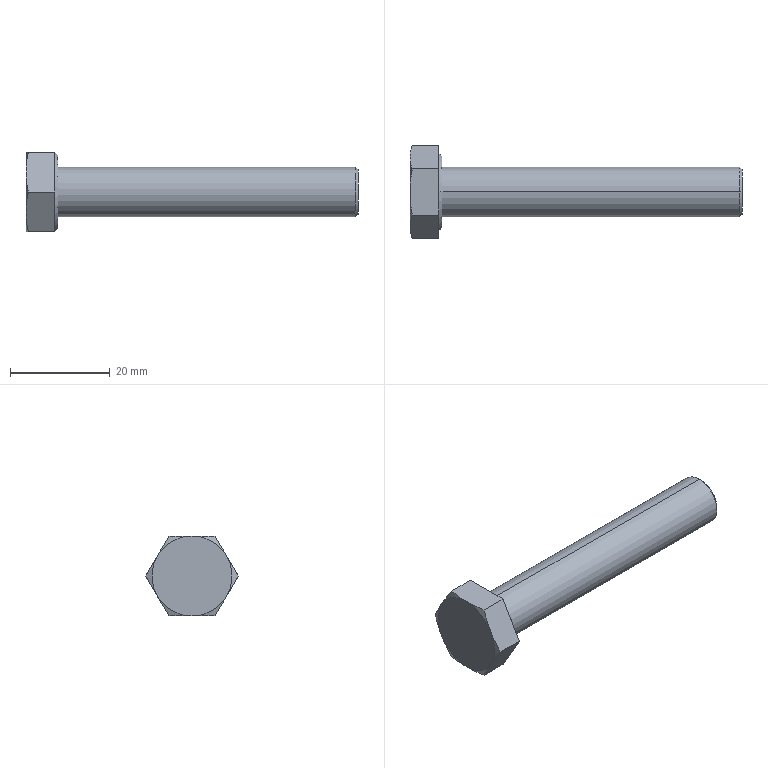Part | SolidWorks | features BaseBody 1 | 1 solid | 22 faces | box 66.4 x 18.475 x 16 mm | volume 6099 mm3 | cone 10 | plane 10 | cylinder 2 | commonest cylinder face diameters 10 x2
STEP:
#1=CARTESIAN_POINT('',(65.9,0.,5.));
#2=VERTEX_POINT('',#1);
#3=CARTESIAN_POINT('',(65.9,0.,-5.));
#4=VERTEX_POINT('',#3);
#5=CARTESIAN_POINT('',(65.9,0.,0.));
#6=DIRECTION('',(-1.,0.,0.));
#7=DIRECTION('',(0.,0.,1.));
#8=AXIS2_PLACEMENT_3D('',#5,#6,#7);
#9=CIRCLE('',#8,5.);
#10=EDGE_CURVE('',#2,#4,#9,.T.);
#11=ORIENTED_EDGE('',*,*,#10,.T.);
#12=CARTESIAN_POINT('',(6.4,0.,-5.));
#13=VERTEX_POINT('',#12);
#14=CARTESIAN_POINT('',(66.4,0.,-5.));
#15=DIRECTION('',(-1.,0.,0.));
#16=VECTOR('',#15,1000.);
#17=LINE('',#14,#16);
#18=EDGE_CURVE('',#4,#13,#17,.T.);
#19=ORIENTED_EDGE('',*,*,#18,.T.);
#20=CARTESIAN_POINT('',(6.4,0.,5.));
#21=VERTEX_POINT('',#20);
#22=CARTESIAN_POINT('',(6.4,0.,0.));
#23=DIRECTION('',(1.,0.,0.));
#24=DIRECTION('',(0.,0.,1.));
#25=AXIS2_PLACEMENT_3D('',#22,#23,#24);
#26=CIRCLE('',#25,5.);
#27=EDGE_CURVE('',#13,#21,#26,.T.);
#28=ORIENTED_EDGE('',*,*,#27,.T.);
#29=CARTESIAN_POINT('',(66.4,0.,5.));
#30=DIRECTION('',(-1.,0.,0.));
#31=VECTOR('',#30,1000.);
#32=LINE('',#29,#31);
#33=EDGE_CURVE('',#2,#21,#32,.T.);
#34=ORIENTED_EDGE('',*,*,#33,.F.);
#35=EDGE_LOOP('',(#11,#19,#28,#34));
#36=FACE_OUTER_BOUND('',#35,.T.);
#37=CARTESIAN_POINT('',(66.4,0.,0.));
#38=DIRECTION('',(-1.,0.,0.));
#39=DIRECTION('',(0.,0.,1.));
#40=AXIS2_PLACEMENT_3D('',#37,#38,#39);
#41=CYLINDRICAL_SURFACE('',#40,5.);
#42=ADVANCED_FACE('',(#36),#41,.T.);
#43=CARTESIAN_POINT('',(66.4,0.,4.5));
#44=VERTEX_POINT('',#43);
#45=CARTESIAN_POINT('',(66.4,0.,-4.5));
#46=VERTEX_POINT('',#45);
#47=CARTESIAN_POINT('',(66.4,0.,0.));
#48=DIRECTION('',(-1.,0.,0.));
#49=DIRECTION('',(0.,0.,1.));
#50=AXIS2_PLACEMENT_3D('',#47,#48,#49);
#51=CIRCLE('',#50,4.5);
#52=EDGE_CURVE('',#44,#46,#51,.T.);
#53=ORIENTED_EDGE('',*,*,#52,.T.);
#54=CARTESIAN_POINT('',(65.9,0.,-5.));
#55=DIRECTION('',(-0.7071,0.,-0.7071));
#56=VECTOR('',#55,1000.);
#57=LINE('',#54,#56);
#58=EDGE_CURVE('',#46,#4,#57,.T.);
#59=ORIENTED_EDGE('',*,*,#58,.T.);
#60=ORIENTED_EDGE('',*,*,#10,.F.);
#61=CARTESIAN_POINT('',(65.9,0.,5.));
#62=DIRECTION('',(-0.7071,0.,0.7071));
#63=VECTOR('',#62,1000.);
#64=LINE('',#61,#63);
#65=EDGE_CURVE('',#44,#2,#64,.T.);
#66=ORIENTED_EDGE('',*,*,#65,.F.);
#67=EDGE_LOOP('',(#53,#59,#60,#66));
#68=FACE_OUTER_BOUND('',#67,.T.);
#69=CARTESIAN_POINT('',(65.9,0.,0.));
#70=DIRECTION('',(-1.,0.,0.));
#71=DIRECTION('',(0.,0.,1.));
#72=AXIS2_PLACEMENT_3D('',#69,#70,#71);
#73=CONICAL_SURFACE('',#72,5.,0.7854);
#74=ADVANCED_FACE('',(#68),#73,.T.);
#75=CARTESIAN_POINT('',(6.4,0.,7.235));
#76=VERTEX_POINT('',#75);
#77=CARTESIAN_POINT('',(6.4,0.,-7.235));
#78=VERTEX_POINT('',#77);
#79=CARTESIAN_POINT('',(6.4,0.,0.));
#80=DIRECTION('',(-1.,0.,0.));
#81=DIRECTION('',(0.,0.,1.));
#82=AXIS2_PLACEMENT_3D('',#79,#80,#81);
#83=CIRCLE('',#82,7.235);
#84=EDGE_CURVE('',#76,#78,#83,.T.);
#85=ORIENTED_EDGE('',*,*,#84,.T.);
#86=CARTESIAN_POINT('',(5.8,0.,-7.835));
#87=VERTEX_POINT('',#86);
#88=CARTESIAN_POINT('',(5.8,0.,-7.835));
#89=DIRECTION('',(-0.7071,0.,-0.7071));
#90=VECTOR('',#89,1000.);
#91=LINE('',#88,#90);
#92=EDGE_CURVE('',#78,#87,#91,.T.);
#93=ORIENTED_EDGE('',*,*,#92,.T.);
#94=CARTESIAN_POINT('',(5.8,0.,7.835));
#95=VERTEX_POINT('',#94);
#96=CARTESIAN_POINT('',(5.8,0.,0.));
#97=DIRECTION('',(1.,0.,0.));
#98=DIRECTION('',(0.,0.,1.));
#99=AXIS2_PLACEMENT_3D('',#96,#97,#98);
#100=CIRCLE('',#99,7.835);
#101=EDGE_CURVE('',#87,#95,#100,.T.);
#102=ORIENTED_EDGE('',*,*,#101,.T.);
#103=CARTESIAN_POINT('',(5.8,0.,7.835));
#104=DIRECTION('',(-0.7071,0.,0.7071));
#105=VECTOR('',#104,1000.);
#106=LINE('',#103,#105);
#107=EDGE_CURVE('',#76,#95,#106,.T.);
#108=ORIENTED_EDGE('',*,*,#107,.F.);
#109=EDGE_LOOP('',(#85,#93,#102,#108));
#110=FACE_OUTER_BOUND('',#109,.T.);
#111=CARTESIAN_POINT('',(5.8,0.,0.));
#112=DIRECTION('',(-1.,0.,0.));
#113=DIRECTION('',(0.,0.,1.));
#114=AXIS2_PLACEMENT_3D('',#111,#112,#113);
#115=CONICAL_SURFACE('',#114,7.835,0.7854);
#116=ADVANCED_FACE('',(#110),#115,.T.);
#117=ORIENTED_EDGE('',*,*,#18,.F.);
#118=CARTESIAN_POINT('',(65.9,0.,0.));
#119=DIRECTION('',(-1.,0.,0.));
#120=DIRECTION('',(0.,0.,1.));
#121=AXIS2_PLACEMENT_3D('',#118,#119,#120);
#122=CIRCLE('',#121,5.);
#123=EDGE_CURVE('',#4,#2,#122,.T.);
#124=ORIENTED_EDGE('',*,*,#123,.T.);
#125=ORIENTED_EDGE('',*,*,#33,.T.);
#126=CARTESIAN_POINT('',(6.4,0.,0.));
#127=DIRECTION('',(1.,0.,0.));
#128=DIRECTION('',(0.,0.,1.));
#129=AXIS2_PLACEMENT_3D('',#126,#127,#128);
#130=CIRCLE('',#129,5.);
#131=EDGE_CURVE('',#21,#13,#130,.T.);
#132=ORIENTED_EDGE('',*,*,#131,.T.);
#133=EDGE_LOOP('',(#117,#124,#125,#132));
#134=FACE_OUTER_BOUND('',#133,.T.);
#135=CARTESIAN_POINT('',(66.4,0.,0.));
#136=DIRECTION('',(-1.,0.,0.));
#137=DIRECTION('',(0.,0.,1.));
#138=AXIS2_PLACEMENT_3D('',#135,#136,#137);
#139=CYLINDRICAL_SURFACE('',#138,5.);
#140=ADVANCED_FACE('',(#134),#139,.T.);
#141=ORIENTED_EDGE('',*,*,#131,.F.);
#142=ORIENTED_EDGE('',*,*,#27,.F.);
#143=EDGE_LOOP('',(#141,#142));
#144=FACE_BOUND('',#143,.T.);
#145=ORIENTED_EDGE('',*,*,#84,.F.);
#146=CARTESIAN_POINT('',(6.4,0.,0.));
#147=DIRECTION('',(-1.,0.,0.));
#148=DIRECTION('',(0.,0.,1.));
#149=AXIS2_PLACEMENT_3D('',#146,#147,#148);
#150=CIRCLE('',#149,7.235);
#151=EDGE_CURVE('',#78,#76,#150,.T.);
#152=ORIENTED_EDGE('',*,*,#151,.F.);
#153=EDGE_LOOP('',(#145,#152));
#154=FACE_OUTER_BOUND('',#153,.T.);
#155=CARTESIAN_POINT('',(6.4,-4.619,8.));
#156=DIRECTION('',(-1.,0.,0.));
#157=DIRECTION('',(0.,0.,1.));
#158=AXIS2_PLACEMENT_3D('',#155,#156,#157);
#159=PLANE('',#158);
#160=ADVANCED_FACE('',(#144,#154),#159,.F.);
#161=ORIENTED_EDGE('',*,*,#58,.F.);
#162=CARTESIAN_POINT('',(66.4,0.,0.));
#163=DIRECTION('',(-1.,0.,0.));
#164=DIRECTION('',(0.,0.,1.));
#165=AXIS2_PLACEMENT_3D('',#162,#163,#164);
#166=CIRCLE('',#165,4.5);
#167=EDGE_CURVE('',#46,#44,#166,.T.);
#168=ORIENTED_EDGE('',*,*,#167,.T.);
#169=ORIENTED_EDGE('',*,*,#65,.T.);
#170=ORIENTED_EDGE('',*,*,#123,.F.);
#171=EDGE_LOOP('',(#161,#168,#169,#170));
#172=FACE_OUTER_BOUND('',#171,.T.);
#173=CARTESIAN_POINT('',(65.9,0.,0.));
#174=DIRECTION('',(-1.,0.,0.));
#175=DIRECTION('',(0.,0.,1.));
#176=AXIS2_PLACEMENT_3D('',#173,#174,#175);
#177=CONICAL_SURFACE('',#176,5.,0.7854);
#178=ADVANCED_FACE('',(#172),#177,.T.);
#179=ORIENTED_EDGE('',*,*,#92,.F.);
#180=ORIENTED_EDGE('',*,*,#151,.T.);
#181=ORIENTED_EDGE('',*,*,#107,.T.);
#182=CARTESIAN_POINT('',(5.8,0.,0.));
#183=DIRECTION('',(1.,0.,0.));
#184=DIRECTION('',(0.,0.,1.));
#185=AXIS2_PLACEMENT_3D('',#182,#183,#184);
#186=CIRCLE('',#185,7.835);
#187=EDGE_CURVE('',#95,#87,#186,.T.);
#188=ORIENTED_EDGE('',*,*,#187,.T.);
#189=EDGE_LOOP('',(#179,#180,#181,#188));
#190=FACE_OUTER_BOUND('',#189,.T.);
#191=CARTESIAN_POINT('',(5.8,0.,0.));
#192=DIRECTION('',(-1.,0.,0.));
#193=DIRECTION('',(0.,0.,1.));
#194=AXIS2_PLACEMENT_3D('',#191,#192,#193);
#195=CONICAL_SURFACE('',#194,7.835,0.7854);
#196=ADVANCED_FACE('',(#190),#195,.T.);
#197=ORIENTED_EDGE('',*,*,#52,.F.);
#198=ORIENTED_EDGE('',*,*,#167,.F.);
#199=EDGE_LOOP('',(#197,#198));
#200=FACE_OUTER_BOUND('',#199,.T.);
#201=CARTESIAN_POINT('',(66.4,0.,0.));
#202=DIRECTION('',(1.,0.,0.));
#203=DIRECTION('',(0.,0.,-1.));
#204=AXIS2_PLACEMENT_3D('',#201,#202,#203);
#205=PLANE('',#204);
#206=ADVANCED_FACE('',(#200),#205,.T.);
#207=CARTESIAN_POINT('',(5.8,9.238,0.));
#208=VERTEX_POINT('',#207);
#209=CARTESIAN_POINT('',(5.8,4.619,8.));
#210=VERTEX_POINT('',#209);
#211=CARTESIAN_POINT('',(5.8,9.238,0.));
#212=DIRECTION('',(0.,-0.5,0.866));
#213=VECTOR('',#212,1000.);
#214=LINE('',#211,#213);
#215=EDGE_CURVE('',#208,#210,#214,.T.);
#216=ORIENTED_EDGE('',*,*,#215,.T.);
#217=CARTESIAN_POINT('',(5.8,-4.619,8.));
#218=VERTEX_POINT('',#217);
#219=CARTESIAN_POINT('',(5.8,7.835,8.));
#220=DIRECTION('',(0.,-1.,0.));
#221=VECTOR('',#220,1000.);
#222=LINE('',#219,#221);
#223=EDGE_CURVE('',#210,#218,#222,.T.);
#224=ORIENTED_EDGE('',*,*,#223,.T.);
#225=CARTESIAN_POINT('',(5.8,-9.238,0.));
#226=VERTEX_POINT('',#225);
#227=CARTESIAN_POINT('',(5.8,-4.619,8.));
#228=DIRECTION('',(0.,-0.5,-0.866));
#229=VECTOR('',#228,1000.);
#230=LINE('',#227,#229);
#231=EDGE_CURVE('',#218,#226,#230,.T.);
#232=ORIENTED_EDGE('',*,*,#231,.T.);
#233=CARTESIAN_POINT('',(5.8,-4.619,-8.));
#234=VERTEX_POINT('',#233);
#235=CARTESIAN_POINT('',(5.8,-9.238,0.));
#236=DIRECTION('',(0.,0.5,-0.866));
#237=VECTOR('',#236,1000.);
#238=LINE('',#235,#237);
#239=EDGE_CURVE('',#226,#234,#238,.T.);
#240=ORIENTED_EDGE('',*,*,#239,.T.);
#241=CARTESIAN_POINT('',(5.8,4.619,-8.));
#242=VERTEX_POINT('',#241);
#243=CARTESIAN_POINT('',(5.8,7.835,-8.));
#244=DIRECTION('',(0.,1.,0.));
#245=VECTOR('',#244,1000.);
#246=LINE('',#243,#245);
#247=EDGE_CURVE('',#234,#242,#246,.T.);
#248=ORIENTED_EDGE('',*,*,#247,.T.);
#249=CARTESIAN_POINT('',(5.8,4.619,-8.));
#250=DIRECTION('',(0.,0.5,0.866));
#251=VECTOR('',#250,1000.);
#252=LINE('',#249,#251);
#253=EDGE_CURVE('',#242,#208,#252,.T.);
#254=ORIENTED_EDGE('',*,*,#253,.T.);
#255=EDGE_LOOP('',(#216,#224,#232,#240,#248,#254));
#256=FACE_OUTER_BOUND('',#255,.T.);
#257=ORIENTED_EDGE('',*,*,#187,.F.);
#258=ORIENTED_EDGE('',*,*,#101,.F.);
#259=EDGE_LOOP('',(#257,#258));
#260=FACE_BOUND('',#259,.T.);
#261=CARTESIAN_POINT('',(5.8,7.835,0.));
#262=DIRECTION('',(1.,0.,0.));
#263=DIRECTION('',(0.,0.,-1.));
#264=AXIS2_PLACEMENT_3D('',#261,#262,#263);
#265=PLANE('',#264);
#266=ADVANCED_FACE('',(#256,#260),#265,.T.);
#267=CARTESIAN_POINT('',(0.4505,-4.619,8.));
#268=VERTEX_POINT('',#267);
#269=CARTESIAN_POINT('',(6.4,-4.619,8.));
#270=DIRECTION('',(-1.,0.,0.));
#271=VECTOR('',#270,1000.);
#272=LINE('',#269,#271);
#273=EDGE_CURVE('',#218,#268,#272,.T.);
#274=ORIENTED_EDGE('',*,*,#273,.F.);
#275=ORIENTED_EDGE('',*,*,#223,.F.);
#276=CARTESIAN_POINT('',(0.4505,4.619,8.));
#277=VERTEX_POINT('',#276);
#278=CARTESIAN_POINT('',(6.4,4.619,8.));
#279=DIRECTION('',(1.,0.,0.));
#280=VECTOR('',#279,1000.);
#281=LINE('',#278,#280);
#282=EDGE_CURVE('',#277,#210,#281,.T.);
#283=ORIENTED_EDGE('',*,*,#282,.F.);
#284=CARTESIAN_POINT('',(0.,0.,8.));
#285=VERTEX_POINT('',#284);
#286=CARTESIAN_POINT('',(0.,0.,8.));
#287=CARTESIAN_POINT('',(0.,0.7771,8.));
#288=CARTESIAN_POINT('',(0.04194,1.55,8.));
#289=CARTESIAN_POINT('',(0.1979,3.089,8.));
#290=CARTESIAN_POINT('',(0.3115,3.855,8.));
#291=CARTESIAN_POINT('',(0.4505,4.619,8.));
#292=B_SPLINE_CURVE_WITH_KNOTS('',3,(#286,#287,#288,#289,#290,#291),.UNSPECIFIED.,.F.,.F.,(4,2,4),(0.,0.00232,0.004641),.UNSPECIFIED.);
#293=EDGE_CURVE('',#285,#277,#292,.T.);
#294=ORIENTED_EDGE('',*,*,#293,.F.);
#295=CARTESIAN_POINT('',(0.4505,-4.619,8.));
#296=CARTESIAN_POINT('',(0.3115,-3.855,8.));
#297=CARTESIAN_POINT('',(0.1979,-3.089,8.));
#298=CARTESIAN_POINT('',(0.04194,-1.55,8.));
#299=CARTESIAN_POINT('',(0.,-0.7771,8.));
#300=CARTESIAN_POINT('',(0.,0.,8.));
#301=B_SPLINE_CURVE_WITH_KNOTS('',3,(#295,#296,#297,#298,#299,#300),.UNSPECIFIED.,.F.,.F.,(4,2,4),(0.,0.00232,0.004641),.UNSPECIFIED.);
#302=EDGE_CURVE('',#268,#285,#301,.T.);
#303=ORIENTED_EDGE('',*,*,#302,.F.);
#304=EDGE_LOOP('',(#274,#275,#283,#294,#303));
#305=FACE_OUTER_BOUND('',#304,.T.);
#306=CARTESIAN_POINT('',(6.4,4.619,8.));
#307=DIRECTION('',(0.,0.,-1.));
#308=DIRECTION('',(-1.,0.,0.));
#309=AXIS2_PLACEMENT_3D('',#306,#307,#308);
#310=PLANE('',#309);
#311=ADVANCED_FACE('',(#305),#310,.F.);
#312=ORIENTED_EDGE('',*,*,#282,.T.);
#313=ORIENTED_EDGE('',*,*,#215,.F.);
#314=CARTESIAN_POINT('',(0.4505,9.238,0.));
#315=VERTEX_POINT('',#314);
#316=CARTESIAN_POINT('',(6.4,9.238,0.));
#317=DIRECTION('',(1.,0.,0.));
#318=VECTOR('',#317,1000.);
#319=LINE('',#316,#318);
#320=EDGE_CURVE('',#315,#208,#319,.T.);
#321=ORIENTED_EDGE('',*,*,#320,.F.);
#322=CARTESIAN_POINT('',(0.,6.928,4.));
#323=VERTEX_POINT('',#322);
#324=CARTESIAN_POINT('',(0.,6.928,4.));
#325=CARTESIAN_POINT('',(0.,7.317,3.327));
#326=CARTESIAN_POINT('',(0.04194,7.703,2.658));
#327=CARTESIAN_POINT('',(0.1979,8.473,1.325));
#328=CARTESIAN_POINT('',(0.3115,8.856,0.6613));
#329=CARTESIAN_POINT('',(0.4505,9.238,0.));
#330=B_SPLINE_CURVE_WITH_KNOTS('',3,(#324,#325,#326,#327,#328,#329),.UNSPECIFIED.,.F.,.F.,(4,2,4),(0.,0.00232,0.004641),.UNSPECIFIED.);
#331=EDGE_CURVE('',#323,#315,#330,.T.);
#332=ORIENTED_EDGE('',*,*,#331,.F.);
#333=CARTESIAN_POINT('',(0.4505,4.619,8.));
#334=CARTESIAN_POINT('',(0.3115,5.001,7.339));
#335=CARTESIAN_POINT('',(0.1979,5.384,6.675));
#336=CARTESIAN_POINT('',(0.04194,6.153,5.342));
#337=CARTESIAN_POINT('',(0.,6.54,4.673));
#338=CARTESIAN_POINT('',(0.,6.928,4.));
#339=B_SPLINE_CURVE_WITH_KNOTS('',3,(#333,#334,#335,#336,#337,#338),.UNSPECIFIED.,.F.,.F.,(4,2,4),(0.,0.00232,0.004641),.UNSPECIFIED.);
#340=EDGE_CURVE('',#277,#323,#339,.T.);
#341=ORIENTED_EDGE('',*,*,#340,.F.);
#342=EDGE_LOOP('',(#312,#313,#321,#332,#341));
#343=FACE_OUTER_BOUND('',#342,.T.);
#344=CARTESIAN_POINT('',(6.4,9.238,0.));
#345=DIRECTION('',(0.,-0.866,-0.5));
#346=DIRECTION('',(0.,0.5,-0.866));
#347=AXIS2_PLACEMENT_3D('',#344,#345,#346);
#348=PLANE('',#347);
#349=ADVANCED_FACE('',(#343),#348,.F.);
#350=ORIENTED_EDGE('',*,*,#320,.T.);
#351=ORIENTED_EDGE('',*,*,#253,.F.);
#352=CARTESIAN_POINT('',(0.4505,4.619,-8.));
#353=VERTEX_POINT('',#352);
#354=CARTESIAN_POINT('',(6.4,4.619,-8.));
#355=DIRECTION('',(1.,0.,0.));
#356=VECTOR('',#355,1000.);
#357=LINE('',#354,#356);
#358=EDGE_CURVE('',#353,#242,#357,.T.);
#359=ORIENTED_EDGE('',*,*,#358,.F.);
#360=CARTESIAN_POINT('',(0.,6.928,-4.));
#361=VERTEX_POINT('',#360);
#362=CARTESIAN_POINT('',(0.,6.928,-4.));
#363=CARTESIAN_POINT('',(0.,6.54,-4.673));
#364=CARTESIAN_POINT('',(0.04194,6.153,-5.342));
#365=CARTESIAN_POINT('',(0.1979,5.384,-6.675));
#366=CARTESIAN_POINT('',(0.3115,5.001,-7.339));
#367=CARTESIAN_POINT('',(0.4505,4.619,-8.));
#368=B_SPLINE_CURVE_WITH_KNOTS('',3,(#362,#363,#364,#365,#366,#367),.UNSPECIFIED.,.F.,.F.,(4,2,4),(0.,0.00232,0.004641),.UNSPECIFIED.);
#369=EDGE_CURVE('',#361,#353,#368,.T.);
#370=ORIENTED_EDGE('',*,*,#369,.F.);
#371=CARTESIAN_POINT('',(0.4505,9.238,0.));
#372=CARTESIAN_POINT('',(0.3115,8.856,-0.6613));
#373=CARTESIAN_POINT('',(0.1979,8.473,-1.325));
#374=CARTESIAN_POINT('',(0.04194,7.703,-2.658));
#375=CARTESIAN_POINT('',(0.,7.317,-3.327));
#376=CARTESIAN_POINT('',(0.,6.928,-4.));
#377=B_SPLINE_CURVE_WITH_KNOTS('',3,(#371,#372,#373,#374,#375,#376),.UNSPECIFIED.,.F.,.F.,(4,2,4),(0.,0.00232,0.004641),.UNSPECIFIED.);
#378=EDGE_CURVE('',#315,#361,#377,.T.);
#379=ORIENTED_EDGE('',*,*,#378,.F.);
#380=EDGE_LOOP('',(#350,#351,#359,#370,#379));
#381=FACE_OUTER_BOUND('',#380,.T.);
#382=CARTESIAN_POINT('',(6.4,4.619,-8.));
#383=DIRECTION('',(0.,-0.866,0.5));
#384=DIRECTION('',(0.,-0.5,-0.866));
#385=AXIS2_PLACEMENT_3D('',#382,#383,#384);
#386=PLANE('',#385);
#387=ADVANCED_FACE('',(#381),#386,.F.);
#388=ORIENTED_EDGE('',*,*,#358,.T.);
#389=ORIENTED_EDGE('',*,*,#247,.F.);
#390=CARTESIAN_POINT('',(0.4505,-4.619,-8.));
#391=VERTEX_POINT('',#390);
#392=CARTESIAN_POINT('',(6.4,-4.619,-8.));
#393=DIRECTION('',(1.,0.,0.));
#394=VECTOR('',#393,1000.);
#395=LINE('',#392,#394);
#396=EDGE_CURVE('',#391,#234,#395,.T.);
#397=ORIENTED_EDGE('',*,*,#396,.F.);
#398=CARTESIAN_POINT('',(0.,0.,-8.));
#399=VERTEX_POINT('',#398);
#400=CARTESIAN_POINT('',(0.,0.,-8.));
#401=CARTESIAN_POINT('',(0.,-0.7771,-8.));
#402=CARTESIAN_POINT('',(0.04194,-1.55,-8.));
#403=CARTESIAN_POINT('',(0.1979,-3.089,-8.));
#404=CARTESIAN_POINT('',(0.3115,-3.855,-8.));
#405=CARTESIAN_POINT('',(0.4505,-4.619,-8.));
#406=B_SPLINE_CURVE_WITH_KNOTS('',3,(#400,#401,#402,#403,#404,#405),.UNSPECIFIED.,.F.,.F.,(4,2,4),(0.,0.00232,0.004641),.UNSPECIFIED.);
#407=EDGE_CURVE('',#399,#391,#406,.T.);
#408=ORIENTED_EDGE('',*,*,#407,.F.);
#409=CARTESIAN_POINT('',(0.4505,4.619,-8.));
#410=CARTESIAN_POINT('',(0.3115,3.855,-8.));
#411=CARTESIAN_POINT('',(0.1979,3.089,-8.));
#412=CARTESIAN_POINT('',(0.04194,1.55,-8.));
#413=CARTESIAN_POINT('',(0.,0.7771,-8.));
#414=CARTESIAN_POINT('',(0.,0.,-8.));
#415=B_SPLINE_CURVE_WITH_KNOTS('',3,(#409,#410,#411,#412,#413,#414),.UNSPECIFIED.,.F.,.F.,(4,2,4),(0.,0.00232,0.004641),.UNSPECIFIED.);
#416=EDGE_CURVE('',#353,#399,#415,.T.);
#417=ORIENTED_EDGE('',*,*,#416,.F.);
#418=EDGE_LOOP('',(#388,#389,#397,#408,#417));
#419=FACE_OUTER_BOUND('',#418,.T.);
#420=CARTESIAN_POINT('',(6.4,-4.619,-8.));
#421=DIRECTION('',(0.,0.,1.));
#422=DIRECTION('',(1.,0.,0.));
#423=AXIS2_PLACEMENT_3D('',#420,#421,#422);
#424=PLANE('',#423);
#425=ADVANCED_FACE('',(#419),#424,.F.);
#426=ORIENTED_EDGE('',*,*,#396,.T.);
#427=ORIENTED_EDGE('',*,*,#239,.F.);
#428=CARTESIAN_POINT('',(0.4505,-9.238,0.));
#429=VERTEX_POINT('',#428);
#430=CARTESIAN_POINT('',(6.4,-9.238,0.));
#431=DIRECTION('',(1.,0.,0.));
#432=VECTOR('',#431,1000.);
#433=LINE('',#430,#432);
#434=EDGE_CURVE('',#429,#226,#433,.T.);
#435=ORIENTED_EDGE('',*,*,#434,.F.);
#436=CARTESIAN_POINT('',(0.,-6.928,-4.));
#437=VERTEX_POINT('',#436);
#438=CARTESIAN_POINT('',(0.,-6.928,-4.));
#439=CARTESIAN_POINT('',(0.,-7.317,-3.327));
#440=CARTESIAN_POINT('',(0.04194,-7.703,-2.658));
#441=CARTESIAN_POINT('',(0.1979,-8.473,-1.325));
#442=CARTESIAN_POINT('',(0.3115,-8.856,-0.6613));
#443=CARTESIAN_POINT('',(0.4505,-9.238,0.));
#444=B_SPLINE_CURVE_WITH_KNOTS('',3,(#438,#439,#440,#441,#442,#443),.UNSPECIFIED.,.F.,.F.,(4,2,4),(0.,0.00232,0.004641),.UNSPECIFIED.);
#445=EDGE_CURVE('',#437,#429,#444,.T.);
#446=ORIENTED_EDGE('',*,*,#445,.F.);
#447=CARTESIAN_POINT('',(0.4505,-4.619,-8.));
#448=CARTESIAN_POINT('',(0.3115,-5.001,-7.339));
#449=CARTESIAN_POINT('',(0.1979,-5.384,-6.675));
#450=CARTESIAN_POINT('',(0.04194,-6.153,-5.342));
#451=CARTESIAN_POINT('',(0.,-6.54,-4.673));
#452=CARTESIAN_POINT('',(0.,-6.928,-4.));
#453=B_SPLINE_CURVE_WITH_KNOTS('',3,(#447,#448,#449,#450,#451,#452),.UNSPECIFIED.,.F.,.F.,(4,2,4),(0.,0.00232,0.004641),.UNSPECIFIED.);
#454=EDGE_CURVE('',#391,#437,#453,.T.);
#455=ORIENTED_EDGE('',*,*,#454,.F.);
#456=EDGE_LOOP('',(#426,#427,#435,#446,#455));
#457=FACE_OUTER_BOUND('',#456,.T.);
#458=CARTESIAN_POINT('',(6.4,-9.238,0.));
#459=DIRECTION('',(0.,0.866,0.5));
#460=DIRECTION('',(0.,-0.5,0.866));
#461=AXIS2_PLACEMENT_3D('',#458,#459,#460);
#462=PLANE('',#461);
#463=ADVANCED_FACE('',(#457),#462,.F.);
#464=ORIENTED_EDGE('',*,*,#434,.T.);
#465=ORIENTED_EDGE('',*,*,#231,.F.);
#466=ORIENTED_EDGE('',*,*,#273,.T.);
#467=CARTESIAN_POINT('',(0.,-6.928,4.));
#468=VERTEX_POINT('',#467);
#469=CARTESIAN_POINT('',(0.,-6.928,4.));
#470=CARTESIAN_POINT('',(0.,-6.54,4.673));
#471=CARTESIAN_POINT('',(0.04194,-6.153,5.342));
#472=CARTESIAN_POINT('',(0.1979,-5.384,6.675));
#473=CARTESIAN_POINT('',(0.3115,-5.001,7.339));
#474=CARTESIAN_POINT('',(0.4505,-4.619,8.));
#475=B_SPLINE_CURVE_WITH_KNOTS('',3,(#469,#470,#471,#472,#473,#474),.UNSPECIFIED.,.F.,.F.,(4,2,4),(0.,0.00232,0.004641),.UNSPECIFIED.);
#476=EDGE_CURVE('',#468,#268,#475,.T.);
#477=ORIENTED_EDGE('',*,*,#476,.F.);
#478=CARTESIAN_POINT('',(0.4505,-9.238,0.));
#479=CARTESIAN_POINT('',(0.3115,-8.856,0.6613));
#480=CARTESIAN_POINT('',(0.1979,-8.473,1.325));
#481=CARTESIAN_POINT('',(0.04194,-7.703,2.658));
#482=CARTESIAN_POINT('',(0.,-7.317,3.327));
#483=CARTESIAN_POINT('',(0.,-6.928,4.));
#484=B_SPLINE_CURVE_WITH_KNOTS('',3,(#478,#479,#480,#481,#482,#483),.UNSPECIFIED.,.F.,.F.,(4,2,4),(0.,0.00232,0.004641),.UNSPECIFIED.);
#485=EDGE_CURVE('',#429,#468,#484,.T.);
#486=ORIENTED_EDGE('',*,*,#485,.F.);
#487=EDGE_LOOP('',(#464,#465,#466,#477,#486));
#488=FACE_OUTER_BOUND('',#487,.T.);
#489=CARTESIAN_POINT('',(6.4,-4.619,8.));
#490=DIRECTION('',(0.,0.866,-0.5));
#491=DIRECTION('',(0.,0.5,0.866));
#492=AXIS2_PLACEMENT_3D('',#489,#490,#491);
#493=PLANE('',#492);
#494=ADVANCED_FACE('',(#488),#493,.F.);
#495=ORIENTED_EDGE('',*,*,#302,.T.);
#496=CARTESIAN_POINT('',(0.,0.,0.));
#497=DIRECTION('',(1.,0.,0.));
#498=DIRECTION('',(0.,0.,-1.));
#499=AXIS2_PLACEMENT_3D('',#496,#497,#498);
#500=CIRCLE('',#499,8.);
#501=EDGE_CURVE('',#285,#468,#500,.T.);
#502=ORIENTED_EDGE('',*,*,#501,.T.);
#503=ORIENTED_EDGE('',*,*,#476,.T.);
#504=EDGE_LOOP('',(#495,#502,#503));
#505=FACE_OUTER_BOUND('',#504,.T.);
#506=CARTESIAN_POINT('',(0.4532,0.,0.));
#507=DIRECTION('',(1.,0.,0.));
#508=DIRECTION('',(0.,0.,-1.));
#509=AXIS2_PLACEMENT_3D('',#506,#507,#508);
#510=CONICAL_SURFACE('',#509,9.245,1.222);
#511=ADVANCED_FACE('',(#505),#510,.T.);
#512=CARTESIAN_POINT('',(0.,0.,0.));
#513=DIRECTION('',(1.,0.,0.));
#514=DIRECTION('',(0.,0.,-1.));
#515=AXIS2_PLACEMENT_3D('',#512,#513,#514);
#516=CIRCLE('',#515,8.);
#517=EDGE_CURVE('',#323,#285,#516,.T.);
#518=ORIENTED_EDGE('',*,*,#517,.T.);
#519=ORIENTED_EDGE('',*,*,#293,.T.);
#520=ORIENTED_EDGE('',*,*,#340,.T.);
#521=EDGE_LOOP('',(#518,#519,#520));
#522=FACE_OUTER_BOUND('',#521,.T.);
#523=CARTESIAN_POINT('',(0.4532,0.,0.));
#524=DIRECTION('',(1.,0.,0.));
#525=DIRECTION('',(0.,0.,-1.));
#526=AXIS2_PLACEMENT_3D('',#523,#524,#525);
#527=CONICAL_SURFACE('',#526,9.245,1.222);
#528=ADVANCED_FACE('',(#522),#527,.T.);
#529=CARTESIAN_POINT('',(0.,0.,0.));
#530=DIRECTION('',(1.,0.,0.));
#531=DIRECTION('',(0.,0.,-1.));
#532=AXIS2_PLACEMENT_3D('',#529,#530,#531);
#533=CIRCLE('',#532,8.);
#534=EDGE_CURVE('',#361,#323,#533,.T.);
#535=ORIENTED_EDGE('',*,*,#534,.T.);
#536=ORIENTED_EDGE('',*,*,#331,.T.);
#537=ORIENTED_EDGE('',*,*,#378,.T.);
#538=EDGE_LOOP('',(#535,#536,#537));
#539=FACE_OUTER_BOUND('',#538,.T.);
#540=CARTESIAN_POINT('',(0.4532,0.,0.));
#541=DIRECTION('',(1.,0.,0.));
#542=DIRECTION('',(0.,0.,-1.));
#543=AXIS2_PLACEMENT_3D('',#540,#541,#542);
#544=CONICAL_SURFACE('',#543,9.245,1.222);
#545=ADVANCED_FACE('',(#539),#544,.T.);
#546=CARTESIAN_POINT('',(0.,0.,0.));
#547=DIRECTION('',(1.,0.,0.));
#548=DIRECTION('',(0.,1.,0.));
#549=AXIS2_PLACEMENT_3D('',#546,#547,#548);
#550=CIRCLE('',#549,8.);
#551=EDGE_CURVE('',#399,#361,#550,.T.);
#552=ORIENTED_EDGE('',*,*,#551,.T.);
#553=ORIENTED_EDGE('',*,*,#369,.T.);
#554=ORIENTED_EDGE('',*,*,#416,.T.);
#555=EDGE_LOOP('',(#552,#553,#554));
#556=FACE_OUTER_BOUND('',#555,.T.);
#557=CARTESIAN_POINT('',(0.4532,0.,0.));
#558=DIRECTION('',(1.,0.,0.));
#559=DIRECTION('',(0.,1.,0.));
#560=AXIS2_PLACEMENT_3D('',#557,#558,#559);
#561=CONICAL_SURFACE('',#560,9.245,1.222);
#562=ADVANCED_FACE('',(#556),#561,.T.);
#563=ORIENTED_EDGE('',*,*,#454,.T.);
#564=CARTESIAN_POINT('',(0.,0.,0.));
#565=DIRECTION('',(1.,0.,0.));
#566=DIRECTION('',(0.,0.,-1.));
#567=AXIS2_PLACEMENT_3D('',#564,#565,#566);
#568=CIRCLE('',#567,8.);
#569=EDGE_CURVE('',#437,#399,#568,.T.);
#570=ORIENTED_EDGE('',*,*,#569,.T.);
#571=ORIENTED_EDGE('',*,*,#407,.T.);
#572=EDGE_LOOP('',(#563,#570,#571));
#573=FACE_OUTER_BOUND('',#572,.T.);
#574=CARTESIAN_POINT('',(0.4532,0.,0.));
#575=DIRECTION('',(1.,0.,0.));
#576=DIRECTION('',(0.,0.,-1.));
#577=AXIS2_PLACEMENT_3D('',#574,#575,#576);
#578=CONICAL_SURFACE('',#577,9.245,1.222);
#579=ADVANCED_FACE('',(#573),#578,.T.);
#580=ORIENTED_EDGE('',*,*,#485,.T.);
#581=CARTESIAN_POINT('',(0.,0.,0.));
#582=DIRECTION('',(1.,0.,0.));
#583=DIRECTION('',(0.,0.,-1.));
#584=AXIS2_PLACEMENT_3D('',#581,#582,#583);
#585=CIRCLE('',#584,8.);
#586=EDGE_CURVE('',#468,#437,#585,.T.);
#587=ORIENTED_EDGE('',*,*,#586,.T.);
#588=ORIENTED_EDGE('',*,*,#445,.T.);
#589=EDGE_LOOP('',(#580,#587,#588));
#590=FACE_OUTER_BOUND('',#589,.T.);
#591=CARTESIAN_POINT('',(0.4532,0.,0.));
#592=DIRECTION('',(1.,0.,0.));
#593=DIRECTION('',(0.,0.,-1.));
#594=AXIS2_PLACEMENT_3D('',#591,#592,#593);
#595=CONICAL_SURFACE('',#594,9.245,1.222);
#596=ADVANCED_FACE('',(#590),#595,.T.);
#597=ORIENTED_EDGE('',*,*,#569,.F.);
#598=ORIENTED_EDGE('',*,*,#586,.F.);
#599=ORIENTED_EDGE('',*,*,#501,.F.);
#600=ORIENTED_EDGE('',*,*,#517,.F.);
#601=ORIENTED_EDGE('',*,*,#534,.F.);
#602=ORIENTED_EDGE('',*,*,#551,.F.);
#603=EDGE_LOOP('',(#597,#598,#599,#600,#601,#602));
#604=FACE_OUTER_BOUND('',#603,.T.);
#605=CARTESIAN_POINT('',(0.,-4.619,8.));
#606=DIRECTION('',(-1.,0.,0.));
#607=DIRECTION('',(0.,0.,1.));
#608=AXIS2_PLACEMENT_3D('',#605,#606,#607);
#609=PLANE('',#608);
#610=ADVANCED_FACE('',(#604),#609,.T.);
#611=CLOSED_SHELL('',(#42,#74,#116,#140,#160,#178,#196,#206,#266,#311,#349,#387,#425,#463,#494,#511,#528,#545,#562,#579,#596,#610));
#612=MANIFOLD_SOLID_BREP('',#611);
#613=CARTESIAN_POINT('',(0.,0.,0.));
#614=DIRECTION('',(0.,0.,1.));
#615=DIRECTION('',(1.,0.,0.));
#616=AXIS2_PLACEMENT_3D('',#613,#614,#615);
#617=(LENGTH_UNIT()NAMED_UNIT(*)SI_UNIT(.MILLI.,.METRE.));
#618=UNCERTAINTY_MEASURE_WITH_UNIT(LENGTH_MEASURE(0.00001),#617,'','');
#619=(NAMED_UNIT(*)PLANE_ANGLE_UNIT()SI_UNIT($,.RADIAN.));
#620=(NAMED_UNIT(*)SI_UNIT($,.STERADIAN.)SOLID_ANGLE_UNIT());
#621=(GEOMETRIC_REPRESENTATION_CONTEXT(3)GLOBAL_UNCERTAINTY_ASSIGNED_CONTEXT((#618))GLOBAL_UNIT_ASSIGNED_CONTEXT((#617,#619,#620))REPRESENTATION_CONTEXT('',''));
#622=ADVANCED_BREP_SHAPE_REPRESENTATION('',(#612,#616),#621);